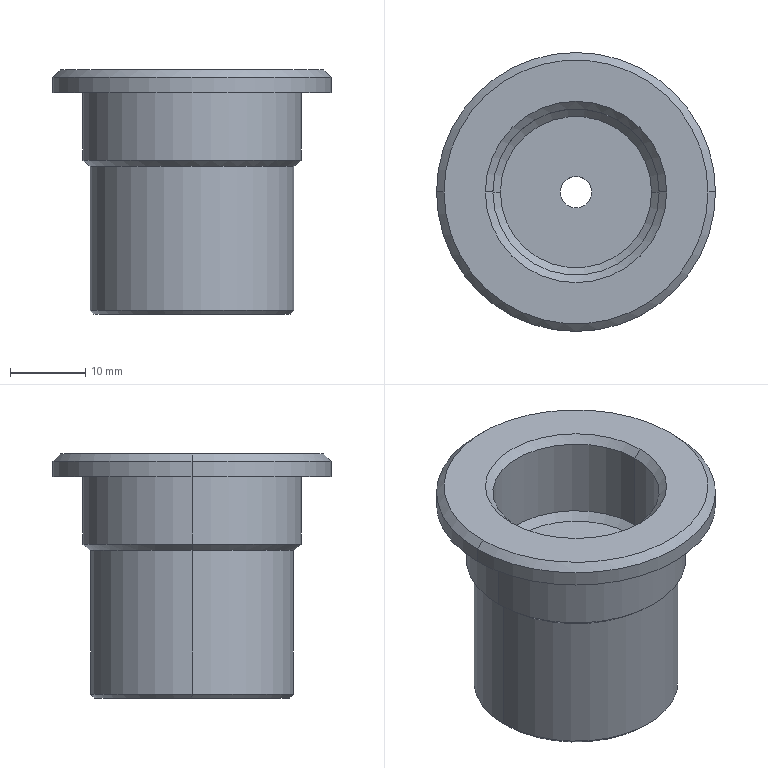Part | SolidWorks | features Chamfer 5, ICE 4, 3DProfileFeature 1, Extrusion 1, HoleWzd 1 | 1 solid | 29 faces | box 37.15 x 37.15 x 32.5 mm | volume 10461 mm3 | cone 12 | cylinder 12 | plane 5 | commonest cylinder face diameters 22.15 x4 4.2 x2 27.15 x2 29.15 x2 37.15 x2
STEP:
#1=CARTESIAN_POINT('',(-13.075,0.,1.));
#2=VERTEX_POINT('',#1);
#3=CARTESIAN_POINT('',(13.075,0.,1.));
#4=VERTEX_POINT('',#3);
#5=CARTESIAN_POINT('',(0.,0.,1.));
#6=DIRECTION('',(0.,0.,-1.));
#7=DIRECTION('',(-1.,0.,0.));
#8=AXIS2_PLACEMENT_3D('',#5,#6,#7);
#9=CIRCLE('',#8,13.075);
#10=EDGE_CURVE('',#2,#4,#9,.T.);
#11=ORIENTED_EDGE('',*,*,#10,.F.);
#12=CARTESIAN_POINT('',(-13.575,0.,1.5));
#13=VERTEX_POINT('',#12);
#14=CARTESIAN_POINT('',(-13.075,0.,1.));
#15=DIRECTION('',(-0.7071,0.,0.7071));
#16=VECTOR('',#15,1000.);
#17=LINE('',#14,#16);
#18=EDGE_CURVE('',#2,#13,#17,.T.);
#19=ORIENTED_EDGE('',*,*,#18,.T.);
#20=CARTESIAN_POINT('',(13.575,0.,1.5));
#21=VERTEX_POINT('',#20);
#22=CARTESIAN_POINT('',(0.,0.,1.5));
#23=DIRECTION('',(0.,0.,1.));
#24=DIRECTION('',(-1.,0.,0.));
#25=AXIS2_PLACEMENT_3D('',#22,#23,#24);
#26=CIRCLE('',#25,13.575);
#27=EDGE_CURVE('',#21,#13,#26,.T.);
#28=ORIENTED_EDGE('',*,*,#27,.F.);
#29=CARTESIAN_POINT('',(13.075,0.,1.));
#30=DIRECTION('',(0.7071,0.,0.7071));
#31=VECTOR('',#30,1000.);
#32=LINE('',#29,#31);
#33=EDGE_CURVE('',#4,#21,#32,.T.);
#34=ORIENTED_EDGE('',*,*,#33,.F.);
#35=EDGE_LOOP('',(#11,#19,#28,#34));
#36=FACE_OUTER_BOUND('',#35,.T.);
#37=CARTESIAN_POINT('',(0.,0.,1.));
#38=DIRECTION('',(0.,0.,1.));
#39=DIRECTION('',(1.,0.,0.));
#40=AXIS2_PLACEMENT_3D('',#37,#38,#39);
#41=CONICAL_SURFACE('',#40,13.075,0.7854);
#42=ADVANCED_FACE('',(#36),#41,.T.);
#43=CARTESIAN_POINT('',(-2.1,0.,15.661));
#44=VERTEX_POINT('',#43);
#45=CARTESIAN_POINT('',(2.1,0.,15.661));
#46=VERTEX_POINT('',#45);
#47=CARTESIAN_POINT('',(0.,0.,15.661));
#48=DIRECTION('',(0.,0.,1.));
#49=DIRECTION('',(1.,0.,0.));
#50=AXIS2_PLACEMENT_3D('',#47,#48,#49);
#51=CIRCLE('',#50,2.1);
#52=EDGE_CURVE('',#44,#46,#51,.T.);
#53=ORIENTED_EDGE('',*,*,#52,.F.);
#54=CARTESIAN_POINT('',(-2.1,0.,20.661));
#55=VERTEX_POINT('',#54);
#56=CARTESIAN_POINT('',(-2.1,0.,20.661));
#57=DIRECTION('',(0.,0.,1.));
#58=VECTOR('',#57,1000.);
#59=LINE('',#56,#58);
#60=EDGE_CURVE('',#44,#55,#59,.T.);
#61=ORIENTED_EDGE('',*,*,#60,.T.);
#62=CARTESIAN_POINT('',(2.1,0.,20.661));
#63=VERTEX_POINT('',#62);
#64=CARTESIAN_POINT('',(0.,0.,20.661));
#65=DIRECTION('',(0.,0.,1.));
#66=DIRECTION('',(1.,0.,0.));
#67=AXIS2_PLACEMENT_3D('',#64,#65,#66);
#68=CIRCLE('',#67,2.1);
#69=EDGE_CURVE('',#55,#63,#68,.T.);
#70=ORIENTED_EDGE('',*,*,#69,.T.);
#71=CARTESIAN_POINT('',(2.1,0.,20.661));
#72=DIRECTION('',(0.,0.,1.));
#73=VECTOR('',#72,1000.);
#74=LINE('',#71,#73);
#75=EDGE_CURVE('',#46,#63,#74,.T.);
#76=ORIENTED_EDGE('',*,*,#75,.F.);
#77=EDGE_LOOP('',(#53,#61,#70,#76));
#78=FACE_OUTER_BOUND('',#77,.T.);
#79=CARTESIAN_POINT('',(0.,0.,20.661));
#80=DIRECTION('',(0.,0.,1.));
#81=DIRECTION('',(1.,0.,0.));
#82=AXIS2_PLACEMENT_3D('',#79,#80,#81);
#83=CYLINDRICAL_SURFACE('',#82,2.1);
#84=ADVANCED_FACE('',(#78),#83,.F.);
#85=CARTESIAN_POINT('',(10.075,0.,15.661));
#86=VERTEX_POINT('',#85);
#87=CARTESIAN_POINT('',(-10.075,0.,15.661));
#88=VERTEX_POINT('',#87);
#89=CARTESIAN_POINT('',(0.,0.,15.661));
#90=DIRECTION('',(0.,0.,-1.));
#91=DIRECTION('',(1.,0.,0.));
#92=AXIS2_PLACEMENT_3D('',#89,#90,#91);
#93=CIRCLE('',#92,10.075);
#94=EDGE_CURVE('',#86,#88,#93,.T.);
#95=ORIENTED_EDGE('',*,*,#94,.F.);
#96=CARTESIAN_POINT('',(11.075,0.,14.661));
#97=VERTEX_POINT('',#96);
#98=CARTESIAN_POINT('',(11.075,0.,14.661));
#99=DIRECTION('',(0.7071,0.,-0.7071));
#100=VECTOR('',#99,1000.);
#101=LINE('',#98,#100);
#102=EDGE_CURVE('',#86,#97,#101,.T.);
#103=ORIENTED_EDGE('',*,*,#102,.T.);
#104=CARTESIAN_POINT('',(-11.075,0.,14.661));
#105=VERTEX_POINT('',#104);
#106=CARTESIAN_POINT('',(0.,0.,14.661));
#107=DIRECTION('',(0.,0.,1.));
#108=DIRECTION('',(1.,0.,0.));
#109=AXIS2_PLACEMENT_3D('',#106,#107,#108);
#110=CIRCLE('',#109,11.075);
#111=EDGE_CURVE('',#105,#97,#110,.T.);
#112=ORIENTED_EDGE('',*,*,#111,.F.);
#113=CARTESIAN_POINT('',(-11.075,0.,14.661));
#114=DIRECTION('',(-0.7071,0.,-0.7071));
#115=VECTOR('',#114,1000.);
#116=LINE('',#113,#115);
#117=EDGE_CURVE('',#88,#105,#116,.T.);
#118=ORIENTED_EDGE('',*,*,#117,.F.);
#119=EDGE_LOOP('',(#95,#103,#112,#118));
#120=FACE_OUTER_BOUND('',#119,.T.);
#121=CARTESIAN_POINT('',(0.,0.,14.661));
#122=DIRECTION('',(0.,0.,-1.));
#123=DIRECTION('',(-1.,0.,0.));
#124=AXIS2_PLACEMENT_3D('',#121,#122,#123);
#125=CONICAL_SURFACE('',#124,11.075,0.7854);
#126=ADVANCED_FACE('',(#120),#125,.F.);
#127=CARTESIAN_POINT('',(-10.075,0.,20.661));
#128=VERTEX_POINT('',#127);
#129=CARTESIAN_POINT('',(10.075,0.,20.661));
#130=VERTEX_POINT('',#129);
#131=CARTESIAN_POINT('',(0.,0.,20.661));
#132=DIRECTION('',(0.,0.,1.));
#133=DIRECTION('',(1.,0.,0.));
#134=AXIS2_PLACEMENT_3D('',#131,#132,#133);
#135=CIRCLE('',#134,10.075);
#136=EDGE_CURVE('',#128,#130,#135,.T.);
#137=ORIENTED_EDGE('',*,*,#136,.F.);
#138=CARTESIAN_POINT('',(-11.075,0.,21.661));
#139=VERTEX_POINT('',#138);
#140=CARTESIAN_POINT('',(-10.075,0.,20.661));
#141=DIRECTION('',(-0.7071,0.,0.7071));
#142=VECTOR('',#141,1000.);
#143=LINE('',#140,#142);
#144=EDGE_CURVE('',#128,#139,#143,.T.);
#145=ORIENTED_EDGE('',*,*,#144,.T.);
#146=CARTESIAN_POINT('',(11.075,0.,21.661));
#147=VERTEX_POINT('',#146);
#148=CARTESIAN_POINT('',(0.,0.,21.661));
#149=DIRECTION('',(0.,0.,-1.));
#150=DIRECTION('',(1.,0.,0.));
#151=AXIS2_PLACEMENT_3D('',#148,#149,#150);
#152=CIRCLE('',#151,11.075);
#153=EDGE_CURVE('',#147,#139,#152,.T.);
#154=ORIENTED_EDGE('',*,*,#153,.F.);
#155=CARTESIAN_POINT('',(10.075,0.,20.661));
#156=DIRECTION('',(0.7071,0.,0.7071));
#157=VECTOR('',#156,1000.);
#158=LINE('',#155,#157);
#159=EDGE_CURVE('',#130,#147,#158,.T.);
#160=ORIENTED_EDGE('',*,*,#159,.F.);
#161=EDGE_LOOP('',(#137,#145,#154,#160));
#162=FACE_OUTER_BOUND('',#161,.T.);
#163=CARTESIAN_POINT('',(0.,0.,20.661));
#164=DIRECTION('',(0.,0.,1.));
#165=DIRECTION('',(1.,0.,0.));
#166=AXIS2_PLACEMENT_3D('',#163,#164,#165);
#167=CONICAL_SURFACE('',#166,10.075,0.7854);
#168=ADVANCED_FACE('',(#162),#167,.F.);
#169=CARTESIAN_POINT('',(-11.075,0.,32.5));
#170=VERTEX_POINT('',#169);
#171=CARTESIAN_POINT('',(11.075,0.,32.5));
#172=VERTEX_POINT('',#171);
#173=CARTESIAN_POINT('',(0.,0.,32.5));
#174=DIRECTION('',(0.,0.,1.));
#175=DIRECTION('',(1.,0.,0.));
#176=AXIS2_PLACEMENT_3D('',#173,#174,#175);
#177=CIRCLE('',#176,11.075);
#178=EDGE_CURVE('',#170,#172,#177,.T.);
#179=ORIENTED_EDGE('',*,*,#178,.F.);
#180=CARTESIAN_POINT('',(-12.075,0.,33.5));
#181=VERTEX_POINT('',#180);
#182=CARTESIAN_POINT('',(-11.075,0.,32.5));
#183=DIRECTION('',(-0.7071,0.,0.7071));
#184=VECTOR('',#183,1000.);
#185=LINE('',#182,#184);
#186=EDGE_CURVE('',#170,#181,#185,.T.);
#187=ORIENTED_EDGE('',*,*,#186,.T.);
#188=CARTESIAN_POINT('',(12.075,0.,33.5));
#189=VERTEX_POINT('',#188);
#190=CARTESIAN_POINT('',(0.,0.,33.5));
#191=DIRECTION('',(0.,0.,-1.));
#192=DIRECTION('',(1.,0.,0.));
#193=AXIS2_PLACEMENT_3D('',#190,#191,#192);
#194=CIRCLE('',#193,12.075);
#195=EDGE_CURVE('',#189,#181,#194,.T.);
#196=ORIENTED_EDGE('',*,*,#195,.F.);
#197=CARTESIAN_POINT('',(11.075,0.,32.5));
#198=DIRECTION('',(0.7071,0.,0.7071));
#199=VECTOR('',#198,1000.);
#200=LINE('',#197,#199);
#201=EDGE_CURVE('',#172,#189,#200,.T.);
#202=ORIENTED_EDGE('',*,*,#201,.F.);
#203=EDGE_LOOP('',(#179,#187,#196,#202));
#204=FACE_OUTER_BOUND('',#203,.T.);
#205=CARTESIAN_POINT('',(0.,0.,32.5));
#206=DIRECTION('',(0.,0.,1.));
#207=DIRECTION('',(1.,0.,0.));
#208=AXIS2_PLACEMENT_3D('',#205,#206,#207);
#209=CONICAL_SURFACE('',#208,11.075,0.7854);
#210=ADVANCED_FACE('',(#204),#209,.F.);
#211=CARTESIAN_POINT('',(17.575,0.,33.5));
#212=VERTEX_POINT('',#211);
#213=CARTESIAN_POINT('',(-17.575,0.,33.5));
#214=VERTEX_POINT('',#213);
#215=CARTESIAN_POINT('',(0.,0.,33.5));
#216=DIRECTION('',(0.,0.,1.));
#217=DIRECTION('',(1.,0.,0.));
#218=AXIS2_PLACEMENT_3D('',#215,#216,#217);
#219=CIRCLE('',#218,17.575);
#220=EDGE_CURVE('',#212,#214,#219,.T.);
#221=ORIENTED_EDGE('',*,*,#220,.F.);
#222=CARTESIAN_POINT('',(18.575,0.,32.5));
#223=VERTEX_POINT('',#222);
#224=CARTESIAN_POINT('',(17.575,0.,33.5));
#225=DIRECTION('',(0.7071,0.,-0.7071));
#226=VECTOR('',#225,1000.);
#227=LINE('',#224,#226);
#228=EDGE_CURVE('',#212,#223,#227,.T.);
#229=ORIENTED_EDGE('',*,*,#228,.T.);
#230=CARTESIAN_POINT('',(-18.575,0.,32.5));
#231=VERTEX_POINT('',#230);
#232=CARTESIAN_POINT('',(0.,0.,32.5));
#233=DIRECTION('',(0.,0.,-1.));
#234=DIRECTION('',(1.,0.,0.));
#235=AXIS2_PLACEMENT_3D('',#232,#233,#234);
#236=CIRCLE('',#235,18.575);
#237=EDGE_CURVE('',#231,#223,#236,.T.);
#238=ORIENTED_EDGE('',*,*,#237,.F.);
#239=CARTESIAN_POINT('',(-17.575,0.,33.5));
#240=DIRECTION('',(-0.7071,0.,-0.7071));
#241=VECTOR('',#240,1000.);
#242=LINE('',#239,#241);
#243=EDGE_CURVE('',#214,#231,#242,.T.);
#244=ORIENTED_EDGE('',*,*,#243,.F.);
#245=EDGE_LOOP('',(#221,#229,#238,#244));
#246=FACE_OUTER_BOUND('',#245,.T.);
#247=CARTESIAN_POINT('',(0.,0.,33.5));
#248=DIRECTION('',(0.,0.,-1.));
#249=DIRECTION('',(-1.,0.,0.));
#250=AXIS2_PLACEMENT_3D('',#247,#248,#249);
#251=CONICAL_SURFACE('',#250,17.575,0.7854);
#252=ADVANCED_FACE('',(#246),#251,.T.);
#253=ORIENTED_EDGE('',*,*,#237,.T.);
#254=CARTESIAN_POINT('',(18.575,0.,30.5));
#255=VERTEX_POINT('',#254);
#256=CARTESIAN_POINT('',(18.575,0.,33.5));
#257=DIRECTION('',(0.,0.,-1.));
#258=VECTOR('',#257,1000.);
#259=LINE('',#256,#258);
#260=EDGE_CURVE('',#223,#255,#259,.T.);
#261=ORIENTED_EDGE('',*,*,#260,.T.);
#262=CARTESIAN_POINT('',(-18.575,0.,30.5));
#263=VERTEX_POINT('',#262);
#264=CARTESIAN_POINT('',(0.,0.,30.5));
#265=DIRECTION('',(0.,0.,1.));
#266=DIRECTION('',(1.,0.,0.));
#267=AXIS2_PLACEMENT_3D('',#264,#265,#266);
#268=CIRCLE('',#267,18.575);
#269=EDGE_CURVE('',#255,#263,#268,.T.);
#270=ORIENTED_EDGE('',*,*,#269,.T.);
#271=CARTESIAN_POINT('',(-18.575,0.,33.5));
#272=DIRECTION('',(0.,0.,-1.));
#273=VECTOR('',#272,1000.);
#274=LINE('',#271,#273);
#275=EDGE_CURVE('',#231,#263,#274,.T.);
#276=ORIENTED_EDGE('',*,*,#275,.F.);
#277=EDGE_LOOP('',(#253,#261,#270,#276));
#278=FACE_OUTER_BOUND('',#277,.T.);
#279=CARTESIAN_POINT('',(0.,0.,33.5));
#280=DIRECTION('',(0.,0.,-1.));
#281=DIRECTION('',(-1.,0.,0.));
#282=AXIS2_PLACEMENT_3D('',#279,#280,#281);
#283=CYLINDRICAL_SURFACE('',#282,18.575);
#284=ADVANCED_FACE('',(#278),#283,.T.);
#285=CARTESIAN_POINT('',(-13.575,0.,20.661));
#286=VERTEX_POINT('',#285);
#287=CARTESIAN_POINT('',(13.575,0.,20.661));
#288=VERTEX_POINT('',#287);
#289=CARTESIAN_POINT('',(0.,0.,20.661));
#290=DIRECTION('',(0.,0.,-1.));
#291=DIRECTION('',(1.,0.,0.));
#292=AXIS2_PLACEMENT_3D('',#289,#290,#291);
#293=CIRCLE('',#292,13.575);
#294=EDGE_CURVE('',#286,#288,#293,.T.);
#295=ORIENTED_EDGE('',*,*,#294,.F.);
#296=CARTESIAN_POINT('',(-14.575,0.,21.5));
#297=VERTEX_POINT('',#296);
#298=CARTESIAN_POINT('',(-14.575,0.,21.5));
#299=DIRECTION('',(-0.766,0.,0.6428));
#300=VECTOR('',#299,1000.);
#301=LINE('',#298,#300);
#302=EDGE_CURVE('',#286,#297,#301,.T.);
#303=ORIENTED_EDGE('',*,*,#302,.T.);
#304=CARTESIAN_POINT('',(14.575,0.,21.5));
#305=VERTEX_POINT('',#304);
#306=CARTESIAN_POINT('',(0.,0.,21.5));
#307=DIRECTION('',(0.,0.,1.));
#308=DIRECTION('',(1.,0.,0.));
#309=AXIS2_PLACEMENT_3D('',#306,#307,#308);
#310=CIRCLE('',#309,14.575);
#311=EDGE_CURVE('',#305,#297,#310,.T.);
#312=ORIENTED_EDGE('',*,*,#311,.F.);
#313=CARTESIAN_POINT('',(14.575,0.,21.5));
#314=DIRECTION('',(0.766,0.,0.6428));
#315=VECTOR('',#314,1000.);
#316=LINE('',#313,#315);
#317=EDGE_CURVE('',#288,#305,#316,.T.);
#318=ORIENTED_EDGE('',*,*,#317,.F.);
#319=EDGE_LOOP('',(#295,#303,#312,#318));
#320=FACE_OUTER_BOUND('',#319,.T.);
#321=CARTESIAN_POINT('',(0.,0.,21.5));
#322=DIRECTION('',(0.,0.,1.));
#323=DIRECTION('',(1.,0.,0.));
#324=AXIS2_PLACEMENT_3D('',#321,#322,#323);
#325=CONICAL_SURFACE('',#324,14.575,0.8727);
#326=ADVANCED_FACE('',(#320),#325,.T.);
#327=CARTESIAN_POINT('',(14.575,0.,30.5));
#328=VERTEX_POINT('',#327);
#329=CARTESIAN_POINT('',(-14.575,0.,30.5));
#330=VERTEX_POINT('',#329);
#331=CARTESIAN_POINT('',(0.,0.,30.5));
#332=DIRECTION('',(0.,0.,1.));
#333=DIRECTION('',(1.,0.,0.));
#334=AXIS2_PLACEMENT_3D('',#331,#332,#333);
#335=CIRCLE('',#334,14.575);
#336=EDGE_CURVE('',#328,#330,#335,.T.);
#337=ORIENTED_EDGE('',*,*,#336,.F.);
#338=CARTESIAN_POINT('',(14.575,0.,30.5));
#339=DIRECTION('',(0.,0.,-1.));
#340=VECTOR('',#339,1000.);
#341=LINE('',#338,#340);
#342=EDGE_CURVE('',#328,#305,#341,.T.);
#343=ORIENTED_EDGE('',*,*,#342,.T.);
#344=ORIENTED_EDGE('',*,*,#311,.T.);
#345=CARTESIAN_POINT('',(-14.575,0.,30.5));
#346=DIRECTION('',(0.,0.,-1.));
#347=VECTOR('',#346,1000.);
#348=LINE('',#345,#347);
#349=EDGE_CURVE('',#330,#297,#348,.T.);
#350=ORIENTED_EDGE('',*,*,#349,.F.);
#351=EDGE_LOOP('',(#337,#343,#344,#350));
#352=FACE_OUTER_BOUND('',#351,.T.);
#353=CARTESIAN_POINT('',(0.,0.,30.5));
#354=DIRECTION('',(0.,0.,-1.));
#355=DIRECTION('',(-1.,0.,0.));
#356=AXIS2_PLACEMENT_3D('',#353,#354,#355);
#357=CYLINDRICAL_SURFACE('',#356,14.575);
#358=ADVANCED_FACE('',(#352),#357,.T.);
#359=ORIENTED_EDGE('',*,*,#178,.T.);
#360=CARTESIAN_POINT('',(11.075,0.,21.5));
#361=DIRECTION('',(0.,0.,-1.));
#362=VECTOR('',#361,1000.);
#363=LINE('',#360,#362);
#364=EDGE_CURVE('',#172,#147,#363,.T.);
#365=ORIENTED_EDGE('',*,*,#364,.T.);
#366=ORIENTED_EDGE('',*,*,#153,.T.);
#367=CARTESIAN_POINT('',(-11.075,0.,21.5));
#368=DIRECTION('',(0.,0.,-1.));
#369=VECTOR('',#368,1000.);
#370=LINE('',#367,#369);
#371=EDGE_CURVE('',#170,#139,#370,.T.);
#372=ORIENTED_EDGE('',*,*,#371,.F.);
#373=EDGE_LOOP('',(#359,#365,#366,#372));
#374=FACE_OUTER_BOUND('',#373,.T.);
#375=CARTESIAN_POINT('',(0.,0.,21.5));
#376=DIRECTION('',(0.,0.,-1.));
#377=DIRECTION('',(-1.,0.,0.));
#378=AXIS2_PLACEMENT_3D('',#375,#376,#377);
#379=CYLINDRICAL_SURFACE('',#378,11.075);
#380=ADVANCED_FACE('',(#374),#379,.F.);
#381=ORIENTED_EDGE('',*,*,#294,.T.);
#382=CARTESIAN_POINT('',(13.575,0.,21.5));
#383=DIRECTION('',(0.,0.,-1.));
#384=VECTOR('',#383,1000.);
#385=LINE('',#382,#384);
#386=EDGE_CURVE('',#288,#21,#385,.T.);
#387=ORIENTED_EDGE('',*,*,#386,.T.);
#388=ORIENTED_EDGE('',*,*,#27,.T.);
#389=CARTESIAN_POINT('',(-13.575,0.,21.5));
#390=DIRECTION('',(0.,0.,-1.));
#391=VECTOR('',#390,1000.);
#392=LINE('',#389,#391);
#393=EDGE_CURVE('',#286,#13,#392,.T.);
#394=ORIENTED_EDGE('',*,*,#393,.F.);
#395=EDGE_LOOP('',(#381,#387,#388,#394));
#396=FACE_OUTER_BOUND('',#395,.T.);
#397=CARTESIAN_POINT('',(0.,0.,21.5));
#398=DIRECTION('',(0.,0.,-1.));
#399=DIRECTION('',(-1.,0.,0.));
#400=AXIS2_PLACEMENT_3D('',#397,#398,#399);
#401=CYLINDRICAL_SURFACE('',#400,13.575);
#402=ADVANCED_FACE('',(#396),#401,.T.);
#403=ORIENTED_EDGE('',*,*,#111,.T.);
#404=CARTESIAN_POINT('',(11.075,0.,1.));
#405=VERTEX_POINT('',#404);
#406=CARTESIAN_POINT('',(11.075,0.,21.5));
#407=DIRECTION('',(0.,0.,-1.));
#408=VECTOR('',#407,1000.);
#409=LINE('',#406,#408);
#410=EDGE_CURVE('',#97,#405,#409,.T.);
#411=ORIENTED_EDGE('',*,*,#410,.T.);
#412=CARTESIAN_POINT('',(-11.075,0.,1.));
#413=VERTEX_POINT('',#412);
#414=CARTESIAN_POINT('',(0.,0.,1.));
#415=DIRECTION('',(0.,0.,-1.));
#416=DIRECTION('',(-1.,0.,0.));
#417=AXIS2_PLACEMENT_3D('',#414,#415,#416);
#418=CIRCLE('',#417,11.075);
#419=EDGE_CURVE('',#405,#413,#418,.T.);
#420=ORIENTED_EDGE('',*,*,#419,.T.);
#421=CARTESIAN_POINT('',(-11.075,0.,21.5));
#422=DIRECTION('',(0.,0.,-1.));
#423=VECTOR('',#422,1000.);
#424=LINE('',#421,#423);
#425=EDGE_CURVE('',#105,#413,#424,.T.);
#426=ORIENTED_EDGE('',*,*,#425,.F.);
#427=EDGE_LOOP('',(#403,#411,#420,#426));
#428=FACE_OUTER_BOUND('',#427,.T.);
#429=CARTESIAN_POINT('',(0.,0.,21.5));
#430=DIRECTION('',(0.,0.,-1.));
#431=DIRECTION('',(-1.,0.,0.));
#432=AXIS2_PLACEMENT_3D('',#429,#430,#431);
#433=CYLINDRICAL_SURFACE('',#432,11.075);
#434=ADVANCED_FACE('',(#428),#433,.F.);
#435=ORIENTED_EDGE('',*,*,#410,.F.);
#436=CARTESIAN_POINT('',(0.,0.,14.661));
#437=DIRECTION('',(0.,0.,1.));
#438=DIRECTION('',(1.,0.,0.));
#439=AXIS2_PLACEMENT_3D('',#436,#437,#438);
#440=CIRCLE('',#439,11.075);
#441=EDGE_CURVE('',#97,#105,#440,.T.);
#442=ORIENTED_EDGE('',*,*,#441,.T.);
#443=ORIENTED_EDGE('',*,*,#425,.T.);
#444=CARTESIAN_POINT('',(0.,0.,1.));
#445=DIRECTION('',(0.,0.,-1.));
#446=DIRECTION('',(-1.,0.,0.));
#447=AXIS2_PLACEMENT_3D('',#444,#445,#446);
#448=CIRCLE('',#447,11.075);
#449=EDGE_CURVE('',#413,#405,#448,.T.);
#450=ORIENTED_EDGE('',*,*,#449,.T.);
#451=EDGE_LOOP('',(#435,#442,#443,#450));
#452=FACE_OUTER_BOUND('',#451,.T.);
#453=CARTESIAN_POINT('',(0.,0.,21.5));
#454=DIRECTION('',(0.,0.,-1.));
#455=DIRECTION('',(-1.,0.,0.));
#456=AXIS2_PLACEMENT_3D('',#453,#454,#455);
#457=CYLINDRICAL_SURFACE('',#456,11.075);
#458=ADVANCED_FACE('',(#452),#457,.F.);
#459=ORIENTED_EDGE('',*,*,#386,.F.);
#460=CARTESIAN_POINT('',(0.,0.,20.661));
#461=DIRECTION('',(0.,0.,-1.));
#462=DIRECTION('',(1.,0.,0.));
#463=AXIS2_PLACEMENT_3D('',#460,#461,#462);
#464=CIRCLE('',#463,13.575);
#465=EDGE_CURVE('',#288,#286,#464,.T.);
#466=ORIENTED_EDGE('',*,*,#465,.T.);
#467=ORIENTED_EDGE('',*,*,#393,.T.);
#468=CARTESIAN_POINT('',(0.,0.,1.5));
#469=DIRECTION('',(0.,0.,1.));
#470=DIRECTION('',(-1.,0.,0.));
#471=AXIS2_PLACEMENT_3D('',#468,#469,#470);
#472=CIRCLE('',#471,13.575);
#473=EDGE_CURVE('',#13,#21,#472,.T.);
#474=ORIENTED_EDGE('',*,*,#473,.T.);
#475=EDGE_LOOP('',(#459,#466,#467,#474));
#476=FACE_OUTER_BOUND('',#475,.T.);
#477=CARTESIAN_POINT('',(0.,0.,21.5));
#478=DIRECTION('',(0.,0.,-1.));
#479=DIRECTION('',(-1.,0.,0.));
#480=AXIS2_PLACEMENT_3D('',#477,#478,#479);
#481=CYLINDRICAL_SURFACE('',#480,13.575);
#482=ADVANCED_FACE('',(#476),#481,.T.);
#483=ORIENTED_EDGE('',*,*,#364,.F.);
#484=CARTESIAN_POINT('',(0.,0.,32.5));
#485=DIRECTION('',(0.,0.,1.));
#486=DIRECTION('',(1.,0.,0.));
#487=AXIS2_PLACEMENT_3D('',#484,#485,#486);
#488=CIRCLE('',#487,11.075);
#489=EDGE_CURVE('',#172,#170,#488,.T.);
#490=ORIENTED_EDGE('',*,*,#489,.T.);
#491=ORIENTED_EDGE('',*,*,#371,.T.);
#492=CARTESIAN_POINT('',(0.,0.,21.661));
#493=DIRECTION('',(0.,0.,-1.));
#494=DIRECTION('',(1.,0.,0.));
#495=AXIS2_PLACEMENT_3D('',#492,#493,#494);
#496=CIRCLE('',#495,11.075);
#497=EDGE_CURVE('',#139,#147,#496,.T.);
#498=ORIENTED_EDGE('',*,*,#497,.T.);
#499=EDGE_LOOP('',(#483,#490,#491,#498));
#500=FACE_OUTER_BOUND('',#499,.T.);
#501=CARTESIAN_POINT('',(0.,0.,21.5));
#502=DIRECTION('',(0.,0.,-1.));
#503=DIRECTION('',(-1.,0.,0.));
#504=AXIS2_PLACEMENT_3D('',#501,#502,#503);
#505=CYLINDRICAL_SURFACE('',#504,11.075);
#506=ADVANCED_FACE('',(#500),#505,.F.);
#507=ORIENTED_EDGE('',*,*,#342,.F.);
#508=CARTESIAN_POINT('',(0.,0.,30.5));
#509=DIRECTION('',(0.,0.,1.));
#510=DIRECTION('',(1.,0.,0.));
#511=AXIS2_PLACEMENT_3D('',#508,#509,#510);
#512=CIRCLE('',#511,14.575);
#513=EDGE_CURVE('',#330,#328,#512,.T.);
#514=ORIENTED_EDGE('',*,*,#513,.F.);
#515=ORIENTED_EDGE('',*,*,#349,.T.);
#516=CARTESIAN_POINT('',(0.,0.,21.5));
#517=DIRECTION('',(0.,0.,1.));
#518=DIRECTION('',(1.,0.,0.));
#519=AXIS2_PLACEMENT_3D('',#516,#517,#518);
#520=CIRCLE('',#519,14.575);
#521=EDGE_CURVE('',#297,#305,#520,.T.);
#522=ORIENTED_EDGE('',*,*,#521,.T.);
#523=EDGE_LOOP('',(#507,#514,#515,#522));
#524=FACE_OUTER_BOUND('',#523,.T.);
#525=CARTESIAN_POINT('',(0.,0.,30.5));
#526=DIRECTION('',(0.,0.,-1.));
#527=DIRECTION('',(-1.,0.,0.));
#528=AXIS2_PLACEMENT_3D('',#525,#526,#527);
#529=CYLINDRICAL_SURFACE('',#528,14.575);
#530=ADVANCED_FACE('',(#524),#529,.T.);
#531=ORIENTED_EDGE('',*,*,#302,.F.);
#532=ORIENTED_EDGE('',*,*,#465,.F.);
#533=ORIENTED_EDGE('',*,*,#317,.T.);
#534=ORIENTED_EDGE('',*,*,#521,.F.);
#535=EDGE_LOOP('',(#531,#532,#533,#534));
#536=FACE_OUTER_BOUND('',#535,.T.);
#537=CARTESIAN_POINT('',(0.,0.,21.5));
#538=DIRECTION('',(0.,0.,1.));
#539=DIRECTION('',(1.,0.,0.));
#540=AXIS2_PLACEMENT_3D('',#537,#538,#539);
#541=CONICAL_SURFACE('',#540,14.575,0.8727);
#542=ADVANCED_FACE('',(#536),#541,.T.);
#543=ORIENTED_EDGE('',*,*,#195,.T.);
#544=CARTESIAN_POINT('',(0.,0.,33.5));
#545=DIRECTION('',(0.,0.,-1.));
#546=DIRECTION('',(1.,0.,0.));
#547=AXIS2_PLACEMENT_3D('',#544,#545,#546);
#548=CIRCLE('',#547,12.075);
#549=EDGE_CURVE('',#181,#189,#548,.T.);
#550=ORIENTED_EDGE('',*,*,#549,.T.);
#551=EDGE_LOOP('',(#543,#550));
#552=FACE_BOUND('',#551,.T.);
#553=CARTESIAN_POINT('',(0.,0.,33.5));
#554=DIRECTION('',(0.,0.,1.));
#555=DIRECTION('',(1.,0.,0.));
#556=AXIS2_PLACEMENT_3D('',#553,#554,#555);
#557=CIRCLE('',#556,17.575);
#558=EDGE_CURVE('',#214,#212,#557,.T.);
#559=ORIENTED_EDGE('',*,*,#558,.T.);
#560=ORIENTED_EDGE('',*,*,#220,.T.);
#561=EDGE_LOOP('',(#559,#560));
#562=FACE_OUTER_BOUND('',#561,.T.);
#563=CARTESIAN_POINT('',(0.,0.,33.5));
#564=DIRECTION('',(0.,0.,1.));
#565=DIRECTION('',(1.,0.,0.));
#566=AXIS2_PLACEMENT_3D('',#563,#564,#565);
#567=PLANE('',#566);
#568=ADVANCED_FACE('',(#552,#562),#567,.T.);
#569=ORIENTED_EDGE('',*,*,#513,.T.);
#570=ORIENTED_EDGE('',*,*,#336,.T.);
#571=EDGE_LOOP('',(#569,#570));
#572=FACE_BOUND('',#571,.T.);
#573=CARTESIAN_POINT('',(0.,0.,30.5));
#574=DIRECTION('',(0.,0.,1.));
#575=DIRECTION('',(1.,0.,0.));
#576=AXIS2_PLACEMENT_3D('',#573,#574,#575);
#577=CIRCLE('',#576,18.575);
#578=EDGE_CURVE('',#263,#255,#577,.T.);
#579=ORIENTED_EDGE('',*,*,#578,.F.);
#580=ORIENTED_EDGE('',*,*,#269,.F.);
#581=EDGE_LOOP('',(#579,#580));
#582=FACE_OUTER_BOUND('',#581,.T.);
#583=CARTESIAN_POINT('',(0.,0.,30.5));
#584=DIRECTION('',(0.,0.,1.));
#585=DIRECTION('',(1.,0.,0.));
#586=AXIS2_PLACEMENT_3D('',#583,#584,#585);
#587=PLANE('',#586);
#588=ADVANCED_FACE('',(#572,#582),#587,.F.);
#589=ORIENTED_EDGE('',*,*,#260,.F.);
#590=CARTESIAN_POINT('',(0.,0.,32.5));
#591=DIRECTION('',(0.,0.,-1.));
#592=DIRECTION('',(1.,0.,0.));
#593=AXIS2_PLACEMENT_3D('',#590,#591,#592);
#594=CIRCLE('',#593,18.575);
#595=EDGE_CURVE('',#223,#231,#594,.T.);
#596=ORIENTED_EDGE('',*,*,#595,.T.);
#597=ORIENTED_EDGE('',*,*,#275,.T.);
#598=ORIENTED_EDGE('',*,*,#578,.T.);
#599=EDGE_LOOP('',(#589,#596,#597,#598));
#600=FACE_OUTER_BOUND('',#599,.T.);
#601=CARTESIAN_POINT('',(0.,0.,33.5));
#602=DIRECTION('',(0.,0.,-1.));
#603=DIRECTION('',(-1.,0.,0.));
#604=AXIS2_PLACEMENT_3D('',#601,#602,#603);
#605=CYLINDRICAL_SURFACE('',#604,18.575);
#606=ADVANCED_FACE('',(#600),#605,.T.);
#607=ORIENTED_EDGE('',*,*,#228,.F.);
#608=ORIENTED_EDGE('',*,*,#558,.F.);
#609=ORIENTED_EDGE('',*,*,#243,.T.);
#610=ORIENTED_EDGE('',*,*,#595,.F.);
#611=EDGE_LOOP('',(#607,#608,#609,#610));
#612=FACE_OUTER_BOUND('',#611,.T.);
#613=CARTESIAN_POINT('',(0.,0.,33.5));
#614=DIRECTION('',(0.,0.,-1.));
#615=DIRECTION('',(-1.,0.,0.));
#616=AXIS2_PLACEMENT_3D('',#613,#614,#615);
#617=CONICAL_SURFACE('',#616,17.575,0.7854);
#618=ADVANCED_FACE('',(#612),#617,.T.);
#619=ORIENTED_EDGE('',*,*,#186,.F.);
#620=ORIENTED_EDGE('',*,*,#489,.F.);
#621=ORIENTED_EDGE('',*,*,#201,.T.);
#622=ORIENTED_EDGE('',*,*,#549,.F.);
#623=EDGE_LOOP('',(#619,#620,#621,#622));
#624=FACE_OUTER_BOUND('',#623,.T.);
#625=CARTESIAN_POINT('',(0.,0.,32.5));
#626=DIRECTION('',(0.,0.,1.));
#627=DIRECTION('',(1.,0.,0.));
#628=AXIS2_PLACEMENT_3D('',#625,#626,#627);
#629=CONICAL_SURFACE('',#628,11.075,0.7854);
#630=ADVANCED_FACE('',(#624),#629,.F.);
#631=CARTESIAN_POINT('',(0.,0.,20.661));
#632=DIRECTION('',(0.,0.,1.));
#633=DIRECTION('',(1.,0.,0.));
#634=AXIS2_PLACEMENT_3D('',#631,#632,#633);
#635=CIRCLE('',#634,2.1);
#636=EDGE_CURVE('',#63,#55,#635,.T.);
#637=ORIENTED_EDGE('',*,*,#636,.F.);
#638=ORIENTED_EDGE('',*,*,#69,.F.);
#639=EDGE_LOOP('',(#637,#638));
#640=FACE_BOUND('',#639,.T.);
#641=CARTESIAN_POINT('',(0.,0.,20.661));
#642=DIRECTION('',(0.,0.,1.));
#643=DIRECTION('',(1.,0.,0.));
#644=AXIS2_PLACEMENT_3D('',#641,#642,#643);
#645=CIRCLE('',#644,10.075);
#646=EDGE_CURVE('',#130,#128,#645,.T.);
#647=ORIENTED_EDGE('',*,*,#646,.T.);
#648=ORIENTED_EDGE('',*,*,#136,.T.);
#649=EDGE_LOOP('',(#647,#648));
#650=FACE_OUTER_BOUND('',#649,.T.);
#651=CARTESIAN_POINT('',(0.,0.,20.661));
#652=DIRECTION('',(0.,0.,1.));
#653=DIRECTION('',(1.,0.,0.));
#654=AXIS2_PLACEMENT_3D('',#651,#652,#653);
#655=PLANE('',#654);
#656=ADVANCED_FACE('',(#640,#650),#655,.T.);
#657=CARTESIAN_POINT('',(0.,0.,15.661));
#658=DIRECTION('',(0.,0.,1.));
#659=DIRECTION('',(1.,0.,0.));
#660=AXIS2_PLACEMENT_3D('',#657,#658,#659);
#661=CIRCLE('',#660,2.1);
#662=EDGE_CURVE('',#46,#44,#661,.T.);
#663=ORIENTED_EDGE('',*,*,#662,.T.);
#664=ORIENTED_EDGE('',*,*,#52,.T.);
#665=EDGE_LOOP('',(#663,#664));
#666=FACE_BOUND('',#665,.T.);
#667=CARTESIAN_POINT('',(0.,0.,15.661));
#668=DIRECTION('',(0.,0.,-1.));
#669=DIRECTION('',(1.,0.,0.));
#670=AXIS2_PLACEMENT_3D('',#667,#668,#669);
#671=CIRCLE('',#670,10.075);
#672=EDGE_CURVE('',#88,#86,#671,.T.);
#673=ORIENTED_EDGE('',*,*,#672,.T.);
#674=ORIENTED_EDGE('',*,*,#94,.T.);
#675=EDGE_LOOP('',(#673,#674));
#676=FACE_OUTER_BOUND('',#675,.T.);
#677=CARTESIAN_POINT('',(0.,0.,15.661));
#678=DIRECTION('',(0.,0.,1.));
#679=DIRECTION('',(1.,0.,0.));
#680=AXIS2_PLACEMENT_3D('',#677,#678,#679);
#681=PLANE('',#680);
#682=ADVANCED_FACE('',(#666,#676),#681,.F.);
#683=ORIENTED_EDGE('',*,*,#144,.F.);
#684=ORIENTED_EDGE('',*,*,#646,.F.);
#685=ORIENTED_EDGE('',*,*,#159,.T.);
#686=ORIENTED_EDGE('',*,*,#497,.F.);
#687=EDGE_LOOP('',(#683,#684,#685,#686));
#688=FACE_OUTER_BOUND('',#687,.T.);
#689=CARTESIAN_POINT('',(0.,0.,20.661));
#690=DIRECTION('',(0.,0.,1.));
#691=DIRECTION('',(1.,0.,0.));
#692=AXIS2_PLACEMENT_3D('',#689,#690,#691);
#693=CONICAL_SURFACE('',#692,10.075,0.7854);
#694=ADVANCED_FACE('',(#688),#693,.F.);
#695=ORIENTED_EDGE('',*,*,#102,.F.);
#696=ORIENTED_EDGE('',*,*,#672,.F.);
#697=ORIENTED_EDGE('',*,*,#117,.T.);
#698=ORIENTED_EDGE('',*,*,#441,.F.);
#699=EDGE_LOOP('',(#695,#696,#697,#698));
#700=FACE_OUTER_BOUND('',#699,.T.);
#701=CARTESIAN_POINT('',(0.,0.,14.661));
#702=DIRECTION('',(0.,0.,-1.));
#703=DIRECTION('',(-1.,0.,0.));
#704=AXIS2_PLACEMENT_3D('',#701,#702,#703);
#705=CONICAL_SURFACE('',#704,11.075,0.7854);
#706=ADVANCED_FACE('',(#700),#705,.F.);
#707=ORIENTED_EDGE('',*,*,#60,.F.);
#708=ORIENTED_EDGE('',*,*,#662,.F.);
#709=ORIENTED_EDGE('',*,*,#75,.T.);
#710=ORIENTED_EDGE('',*,*,#636,.T.);
#711=EDGE_LOOP('',(#707,#708,#709,#710));
#712=FACE_OUTER_BOUND('',#711,.T.);
#713=CARTESIAN_POINT('',(0.,0.,20.661));
#714=DIRECTION('',(0.,0.,1.));
#715=DIRECTION('',(1.,0.,0.));
#716=AXIS2_PLACEMENT_3D('',#713,#714,#715);
#717=CYLINDRICAL_SURFACE('',#716,2.1);
#718=ADVANCED_FACE('',(#712),#717,.F.);
#719=CARTESIAN_POINT('',(0.,0.,1.));
#720=DIRECTION('',(0.,0.,-1.));
#721=DIRECTION('',(-1.,0.,0.));
#722=AXIS2_PLACEMENT_3D('',#719,#720,#721);
#723=CIRCLE('',#722,13.075);
#724=EDGE_CURVE('',#4,#2,#723,.T.);
#725=ORIENTED_EDGE('',*,*,#724,.T.);
#726=ORIENTED_EDGE('',*,*,#10,.T.);
#727=EDGE_LOOP('',(#725,#726));
#728=FACE_OUTER_BOUND('',#727,.T.);
#729=ORIENTED_EDGE('',*,*,#449,.F.);
#730=ORIENTED_EDGE('',*,*,#419,.F.);
#731=EDGE_LOOP('',(#729,#730));
#732=FACE_BOUND('',#731,.T.);
#733=CARTESIAN_POINT('',(0.,0.,1.));
#734=DIRECTION('',(0.,0.,-1.));
#735=DIRECTION('',(-1.,0.,0.));
#736=AXIS2_PLACEMENT_3D('',#733,#734,#735);
#737=PLANE('',#736);
#738=ADVANCED_FACE('',(#728,#732),#737,.T.);
#739=ORIENTED_EDGE('',*,*,#18,.F.);
#740=ORIENTED_EDGE('',*,*,#724,.F.);
#741=ORIENTED_EDGE('',*,*,#33,.T.);
#742=ORIENTED_EDGE('',*,*,#473,.F.);
#743=EDGE_LOOP('',(#739,#740,#741,#742));
#744=FACE_OUTER_BOUND('',#743,.T.);
#745=CARTESIAN_POINT('',(0.,0.,1.));
#746=DIRECTION('',(0.,0.,1.));
#747=DIRECTION('',(1.,0.,0.));
#748=AXIS2_PLACEMENT_3D('',#745,#746,#747);
#749=CONICAL_SURFACE('',#748,13.075,0.7854);
#750=ADVANCED_FACE('',(#744),#749,.T.);
#751=CLOSED_SHELL('',(#42,#84,#126,#168,#210,#252,#284,#326,#358,#380,#402,#434,#458,#482,#506,#530,#542,#568,#588,#606,#618,#630,#656,#682,#694,#706,#718,#738,#750));
#752=MANIFOLD_SOLID_BREP('',#751);
#753=CARTESIAN_POINT('',(0.,0.,0.));
#754=DIRECTION('',(0.,0.,1.));
#755=DIRECTION('',(1.,0.,0.));
#756=AXIS2_PLACEMENT_3D('',#753,#754,#755);
#757=(LENGTH_UNIT()NAMED_UNIT(*)SI_UNIT(.MILLI.,.METRE.));
#758=UNCERTAINTY_MEASURE_WITH_UNIT(LENGTH_MEASURE(0.00001),#757,'','');
#759=(NAMED_UNIT(*)PLANE_ANGLE_UNIT()SI_UNIT($,.RADIAN.));
#760=(NAMED_UNIT(*)SI_UNIT($,.STERADIAN.)SOLID_ANGLE_UNIT());
#761=(GEOMETRIC_REPRESENTATION_CONTEXT(3)GLOBAL_UNCERTAINTY_ASSIGNED_CONTEXT((#758))GLOBAL_UNIT_ASSIGNED_CONTEXT((#757,#759,#760))REPRESENTATION_CONTEXT('',''));
#762=ADVANCED_BREP_SHAPE_REPRESENTATION('',(#752,#756),#761);